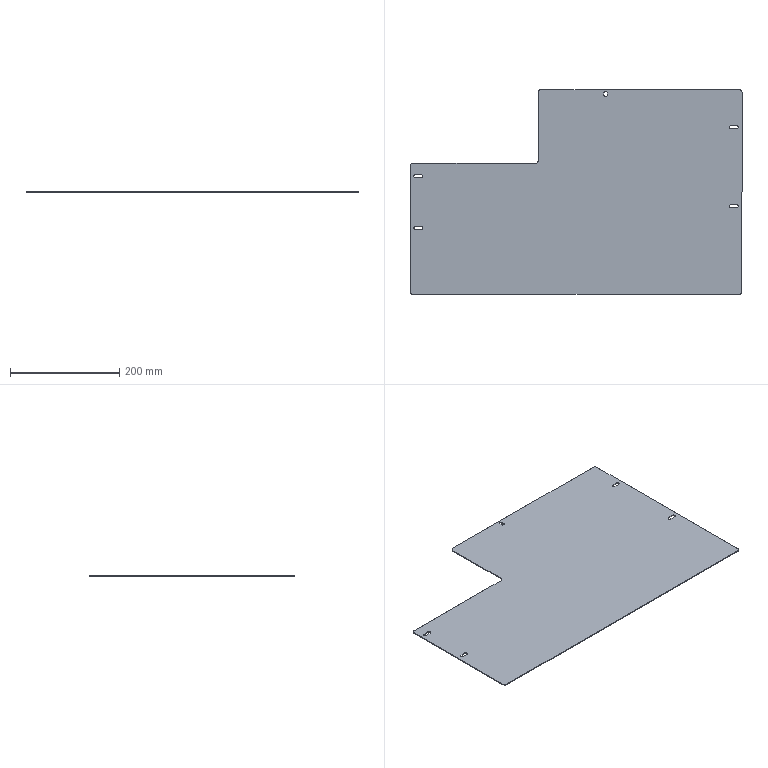Part | SolidWorks | features ICE 3, LPattern 2, FlatPattern 1, SMBaseFlange 1, SheetMetal 1 | 1 solid | 38 faces | box 608.5 x 375 x 1.5 mm | volume 294054 mm3 | cylinder 20 | plane 18 | commonest cylinder face diameters 6 x14 10 x6
STEP:
#1=CARTESIAN_POINT('',(755.768,60.78,-1.5));
#2=VERTEX_POINT('',#1);
#3=CARTESIAN_POINT('',(752.768,63.78,-1.5));
#4=VERTEX_POINT('',#3);
#5=CARTESIAN_POINT('',(752.768,60.78,-1.5));
#6=DIRECTION('',(0.,0.,1.));
#7=DIRECTION('',(1.,0.,0.));
#8=AXIS2_PLACEMENT_3D('',#5,#6,#7);
#9=CIRCLE('',#8,3.);
#10=EDGE_CURVE('',#2,#4,#9,.T.);
#11=ORIENTED_EDGE('',*,*,#10,.F.);
#12=CARTESIAN_POINT('',(755.768,60.78,0.));
#13=VERTEX_POINT('',#12);
#14=CARTESIAN_POINT('',(755.768,60.78,-1.5));
#15=DIRECTION('',(0.,0.,1.));
#16=VECTOR('',#15,1000.);
#17=LINE('',#14,#16);
#18=EDGE_CURVE('',#2,#13,#17,.T.);
#19=ORIENTED_EDGE('',*,*,#18,.T.);
#20=CARTESIAN_POINT('',(752.768,63.78,0.));
#21=VERTEX_POINT('',#20);
#22=CARTESIAN_POINT('',(752.768,60.78,0.));
#23=DIRECTION('',(0.,0.,1.));
#24=DIRECTION('',(1.,0.,0.));
#25=AXIS2_PLACEMENT_3D('',#22,#23,#24);
#26=CIRCLE('',#25,3.);
#27=EDGE_CURVE('',#13,#21,#26,.T.);
#28=ORIENTED_EDGE('',*,*,#27,.T.);
#29=CARTESIAN_POINT('',(752.768,63.78,-1.5));
#30=DIRECTION('',(0.,0.,1.));
#31=VECTOR('',#30,1000.);
#32=LINE('',#29,#31);
#33=EDGE_CURVE('',#4,#21,#32,.T.);
#34=ORIENTED_EDGE('',*,*,#33,.F.);
#35=EDGE_LOOP('',(#11,#19,#28,#34));
#36=FACE_OUTER_BOUND('',#35,.T.);
#37=CARTESIAN_POINT('',(752.768,60.78,-1.5));
#38=DIRECTION('',(0.,0.,1.));
#39=DIRECTION('',(1.,0.,0.));
#40=AXIS2_PLACEMENT_3D('',#37,#38,#39);
#41=CYLINDRICAL_SURFACE('',#40,3.);
#42=ADVANCED_FACE('',(#36),#41,.F.);
#43=CARTESIAN_POINT('',(755.768,205.78,-1.5));
#44=VERTEX_POINT('',#43);
#45=CARTESIAN_POINT('',(752.768,208.78,-1.5));
#46=VERTEX_POINT('',#45);
#47=CARTESIAN_POINT('',(752.768,205.78,-1.5));
#48=DIRECTION('',(0.,0.,1.));
#49=DIRECTION('',(1.,0.,0.));
#50=AXIS2_PLACEMENT_3D('',#47,#48,#49);
#51=CIRCLE('',#50,3.);
#52=EDGE_CURVE('',#44,#46,#51,.T.);
#53=ORIENTED_EDGE('',*,*,#52,.F.);
#54=CARTESIAN_POINT('',(755.768,205.78,0.));
#55=VERTEX_POINT('',#54);
#56=CARTESIAN_POINT('',(755.768,205.78,-1.5));
#57=DIRECTION('',(0.,0.,1.));
#58=VECTOR('',#57,1000.);
#59=LINE('',#56,#58);
#60=EDGE_CURVE('',#44,#55,#59,.T.);
#61=ORIENTED_EDGE('',*,*,#60,.T.);
#62=CARTESIAN_POINT('',(752.768,208.78,0.));
#63=VERTEX_POINT('',#62);
#64=CARTESIAN_POINT('',(752.768,205.78,0.));
#65=DIRECTION('',(0.,0.,1.));
#66=DIRECTION('',(1.,0.,0.));
#67=AXIS2_PLACEMENT_3D('',#64,#65,#66);
#68=CIRCLE('',#67,3.);
#69=EDGE_CURVE('',#55,#63,#68,.T.);
#70=ORIENTED_EDGE('',*,*,#69,.T.);
#71=CARTESIAN_POINT('',(752.768,208.78,-1.5));
#72=DIRECTION('',(0.,0.,1.));
#73=VECTOR('',#72,1000.);
#74=LINE('',#71,#73);
#75=EDGE_CURVE('',#46,#63,#74,.T.);
#76=ORIENTED_EDGE('',*,*,#75,.F.);
#77=EDGE_LOOP('',(#53,#61,#70,#76));
#78=FACE_OUTER_BOUND('',#77,.T.);
#79=CARTESIAN_POINT('',(752.768,205.78,-1.5));
#80=DIRECTION('',(0.,0.,1.));
#81=DIRECTION('',(1.,0.,0.));
#82=AXIS2_PLACEMENT_3D('',#79,#80,#81);
#83=CYLINDRICAL_SURFACE('',#82,3.);
#84=ADVANCED_FACE('',(#78),#83,.F.);
#85=CARTESIAN_POINT('',(174.268,118.78,-1.5));
#86=VERTEX_POINT('',#85);
#87=CARTESIAN_POINT('',(177.268,115.78,-1.5));
#88=VERTEX_POINT('',#87);
#89=CARTESIAN_POINT('',(174.268,115.78,-1.5));
#90=DIRECTION('',(0.,0.,-1.));
#91=DIRECTION('',(-1.,0.,0.));
#92=AXIS2_PLACEMENT_3D('',#89,#90,#91);
#93=CIRCLE('',#92,3.);
#94=EDGE_CURVE('',#86,#88,#93,.T.);
#95=ORIENTED_EDGE('',*,*,#94,.T.);
#96=CARTESIAN_POINT('',(177.268,115.78,0.));
#97=VERTEX_POINT('',#96);
#98=CARTESIAN_POINT('',(177.268,115.78,-10.));
#99=DIRECTION('',(0.,0.,1.));
#100=VECTOR('',#99,1000.);
#101=LINE('',#98,#100);
#102=EDGE_CURVE('',#88,#97,#101,.T.);
#103=ORIENTED_EDGE('',*,*,#102,.T.);
#104=CARTESIAN_POINT('',(174.268,118.78,0.));
#105=VERTEX_POINT('',#104);
#106=CARTESIAN_POINT('',(174.268,115.78,0.));
#107=DIRECTION('',(0.,0.,1.));
#108=DIRECTION('',(1.,0.,0.));
#109=AXIS2_PLACEMENT_3D('',#106,#107,#108);
#110=CIRCLE('',#109,3.);
#111=EDGE_CURVE('',#97,#105,#110,.T.);
#112=ORIENTED_EDGE('',*,*,#111,.T.);
#113=CARTESIAN_POINT('',(174.268,118.78,-10.));
#114=DIRECTION('',(0.,0.,1.));
#115=VECTOR('',#114,1000.);
#116=LINE('',#113,#115);
#117=EDGE_CURVE('',#86,#105,#116,.T.);
#118=ORIENTED_EDGE('',*,*,#117,.F.);
#119=EDGE_LOOP('',(#95,#103,#112,#118));
#120=FACE_OUTER_BOUND('',#119,.T.);
#121=CARTESIAN_POINT('',(174.268,115.78,-10.));
#122=DIRECTION('',(0.,0.,1.));
#123=DIRECTION('',(1.,0.,0.));
#124=AXIS2_PLACEMENT_3D('',#121,#122,#123);
#125=CYLINDRICAL_SURFACE('',#124,3.);
#126=ADVANCED_FACE('',(#120),#125,.F.);
#127=CARTESIAN_POINT('',(174.268,23.78,-1.5));
#128=VERTEX_POINT('',#127);
#129=CARTESIAN_POINT('',(177.268,20.78,-1.5));
#130=VERTEX_POINT('',#129);
#131=CARTESIAN_POINT('',(174.268,20.78,-1.5));
#132=DIRECTION('',(0.,0.,-1.));
#133=DIRECTION('',(-1.,0.,0.));
#134=AXIS2_PLACEMENT_3D('',#131,#132,#133);
#135=CIRCLE('',#134,3.);
#136=EDGE_CURVE('',#128,#130,#135,.T.);
#137=ORIENTED_EDGE('',*,*,#136,.T.);
#138=CARTESIAN_POINT('',(177.268,20.78,0.));
#139=VERTEX_POINT('',#138);
#140=CARTESIAN_POINT('',(177.268,20.78,-10.));
#141=DIRECTION('',(0.,0.,1.));
#142=VECTOR('',#141,1000.);
#143=LINE('',#140,#142);
#144=EDGE_CURVE('',#130,#139,#143,.T.);
#145=ORIENTED_EDGE('',*,*,#144,.T.);
#146=CARTESIAN_POINT('',(174.268,23.78,0.));
#147=VERTEX_POINT('',#146);
#148=CARTESIAN_POINT('',(174.268,20.78,0.));
#149=DIRECTION('',(0.,0.,1.));
#150=DIRECTION('',(1.,0.,0.));
#151=AXIS2_PLACEMENT_3D('',#148,#149,#150);
#152=CIRCLE('',#151,3.);
#153=EDGE_CURVE('',#139,#147,#152,.T.);
#154=ORIENTED_EDGE('',*,*,#153,.T.);
#155=CARTESIAN_POINT('',(174.268,23.78,-10.));
#156=DIRECTION('',(0.,0.,1.));
#157=VECTOR('',#156,1000.);
#158=LINE('',#155,#157);
#159=EDGE_CURVE('',#128,#147,#158,.T.);
#160=ORIENTED_EDGE('',*,*,#159,.F.);
#161=EDGE_LOOP('',(#137,#145,#154,#160));
#162=FACE_OUTER_BOUND('',#161,.T.);
#163=CARTESIAN_POINT('',(174.268,20.78,-10.));
#164=DIRECTION('',(0.,0.,1.));
#165=DIRECTION('',(1.,0.,0.));
#166=AXIS2_PLACEMENT_3D('',#163,#164,#165);
#167=CYLINDRICAL_SURFACE('',#166,3.);
#168=ADVANCED_FACE('',(#162),#167,.F.);
#169=CARTESIAN_POINT('',(389.268,144.28,0.));
#170=VERTEX_POINT('',#169);
#171=CARTESIAN_POINT('',(384.268,139.28,0.));
#172=VERTEX_POINT('',#171);
#173=CARTESIAN_POINT('',(384.268,144.28,0.));
#174=DIRECTION('',(0.,0.,-1.));
#175=DIRECTION('',(-1.,0.,0.));
#176=AXIS2_PLACEMENT_3D('',#173,#174,#175);
#177=CIRCLE('',#176,5.);
#178=EDGE_CURVE('',#170,#172,#177,.T.);
#179=ORIENTED_EDGE('',*,*,#178,.F.);
#180=CARTESIAN_POINT('',(389.268,144.28,-1.5));
#181=VERTEX_POINT('',#180);
#182=CARTESIAN_POINT('',(389.268,144.28,-1.5));
#183=DIRECTION('',(0.,0.,1.));
#184=VECTOR('',#183,1000.);
#185=LINE('',#182,#184);
#186=EDGE_CURVE('',#181,#170,#185,.T.);
#187=ORIENTED_EDGE('',*,*,#186,.F.);
#188=CARTESIAN_POINT('',(384.268,139.28,-1.5));
#189=VERTEX_POINT('',#188);
#190=CARTESIAN_POINT('',(384.268,144.28,-1.5));
#191=DIRECTION('',(0.,0.,-1.));
#192=DIRECTION('',(-1.,0.,0.));
#193=AXIS2_PLACEMENT_3D('',#190,#191,#192);
#194=CIRCLE('',#193,5.);
#195=EDGE_CURVE('',#181,#189,#194,.T.);
#196=ORIENTED_EDGE('',*,*,#195,.T.);
#197=CARTESIAN_POINT('',(384.268,139.28,-1.5));
#198=DIRECTION('',(0.,0.,1.));
#199=VECTOR('',#198,1000.);
#200=LINE('',#197,#199);
#201=EDGE_CURVE('',#189,#172,#200,.T.);
#202=ORIENTED_EDGE('',*,*,#201,.T.);
#203=EDGE_LOOP('',(#179,#187,#196,#202));
#204=FACE_OUTER_BOUND('',#203,.T.);
#205=CARTESIAN_POINT('',(384.268,144.28,-1.5));
#206=DIRECTION('',(0.,0.,1.));
#207=DIRECTION('',(1.,0.,0.));
#208=AXIS2_PLACEMENT_3D('',#205,#206,#207);
#209=CYLINDRICAL_SURFACE('',#208,5.);
#210=ADVANCED_FACE('',(#204),#209,.F.);
#211=CARTESIAN_POINT('',(389.268,269.28,0.));
#212=VERTEX_POINT('',#211);
#213=CARTESIAN_POINT('',(389.268,269.28,0.));
#214=DIRECTION('',(0.,-1.,0.));
#215=VECTOR('',#214,1000.);
#216=LINE('',#213,#215);
#217=EDGE_CURVE('',#212,#170,#216,.T.);
#218=ORIENTED_EDGE('',*,*,#217,.F.);
#219=CARTESIAN_POINT('',(389.268,269.28,-1.5));
#220=VERTEX_POINT('',#219);
#221=CARTESIAN_POINT('',(389.268,269.28,-1.5));
#222=DIRECTION('',(0.,0.,1.));
#223=VECTOR('',#222,1000.);
#224=LINE('',#221,#223);
#225=EDGE_CURVE('',#220,#212,#224,.T.);
#226=ORIENTED_EDGE('',*,*,#225,.F.);
#227=CARTESIAN_POINT('',(389.268,269.28,-1.5));
#228=DIRECTION('',(0.,-1.,0.));
#229=VECTOR('',#228,1000.);
#230=LINE('',#227,#229);
#231=EDGE_CURVE('',#220,#181,#230,.T.);
#232=ORIENTED_EDGE('',*,*,#231,.T.);
#233=ORIENTED_EDGE('',*,*,#186,.T.);
#234=EDGE_LOOP('',(#218,#226,#232,#233));
#235=FACE_OUTER_BOUND('',#234,.T.);
#236=CARTESIAN_POINT('',(389.268,269.28,-1.5));
#237=DIRECTION('',(-1.,0.,0.));
#238=DIRECTION('',(0.,0.,1.));
#239=AXIS2_PLACEMENT_3D('',#236,#237,#238);
#240=PLANE('',#239);
#241=ADVANCED_FACE('',(#235),#240,.T.);
#242=CARTESIAN_POINT('',(394.268,274.28,0.));
#243=VERTEX_POINT('',#242);
#244=CARTESIAN_POINT('',(394.268,269.28,0.));
#245=DIRECTION('',(0.,0.,1.));
#246=DIRECTION('',(-1.,0.,0.));
#247=AXIS2_PLACEMENT_3D('',#244,#245,#246);
#248=CIRCLE('',#247,5.);
#249=EDGE_CURVE('',#243,#212,#248,.T.);
#250=ORIENTED_EDGE('',*,*,#249,.F.);
#251=CARTESIAN_POINT('',(394.268,274.28,-1.5));
#252=VERTEX_POINT('',#251);
#253=CARTESIAN_POINT('',(394.268,274.28,-1.5));
#254=DIRECTION('',(0.,0.,1.));
#255=VECTOR('',#254,1000.);
#256=LINE('',#253,#255);
#257=EDGE_CURVE('',#252,#243,#256,.T.);
#258=ORIENTED_EDGE('',*,*,#257,.F.);
#259=CARTESIAN_POINT('',(394.268,269.28,-1.5));
#260=DIRECTION('',(0.,0.,1.));
#261=DIRECTION('',(-1.,0.,0.));
#262=AXIS2_PLACEMENT_3D('',#259,#260,#261);
#263=CIRCLE('',#262,5.);
#264=EDGE_CURVE('',#252,#220,#263,.T.);
#265=ORIENTED_EDGE('',*,*,#264,.T.);
#266=ORIENTED_EDGE('',*,*,#225,.T.);
#267=EDGE_LOOP('',(#250,#258,#265,#266));
#268=FACE_OUTER_BOUND('',#267,.T.);
#269=CARTESIAN_POINT('',(394.268,269.28,-1.5));
#270=DIRECTION('',(0.,0.,1.));
#271=DIRECTION('',(1.,0.,0.));
#272=AXIS2_PLACEMENT_3D('',#269,#270,#271);
#273=CYLINDRICAL_SURFACE('',#272,5.);
#274=ADVANCED_FACE('',(#268),#273,.T.);
#275=CARTESIAN_POINT('',(757.768,274.28,0.));
#276=VERTEX_POINT('',#275);
#277=CARTESIAN_POINT('',(757.768,274.28,0.));
#278=DIRECTION('',(-1.,0.,0.));
#279=VECTOR('',#278,1000.);
#280=LINE('',#277,#279);
#281=EDGE_CURVE('',#276,#243,#280,.T.);
#282=ORIENTED_EDGE('',*,*,#281,.F.);
#283=CARTESIAN_POINT('',(757.768,274.28,-1.5));
#284=VERTEX_POINT('',#283);
#285=CARTESIAN_POINT('',(757.768,274.28,-1.5));
#286=DIRECTION('',(0.,0.,1.));
#287=VECTOR('',#286,1000.);
#288=LINE('',#285,#287);
#289=EDGE_CURVE('',#284,#276,#288,.T.);
#290=ORIENTED_EDGE('',*,*,#289,.F.);
#291=CARTESIAN_POINT('',(757.768,274.28,-1.5));
#292=DIRECTION('',(-1.,0.,0.));
#293=VECTOR('',#292,1000.);
#294=LINE('',#291,#293);
#295=EDGE_CURVE('',#284,#252,#294,.T.);
#296=ORIENTED_EDGE('',*,*,#295,.T.);
#297=ORIENTED_EDGE('',*,*,#257,.T.);
#298=EDGE_LOOP('',(#282,#290,#296,#297));
#299=FACE_OUTER_BOUND('',#298,.T.);
#300=CARTESIAN_POINT('',(757.768,274.28,-1.5));
#301=DIRECTION('',(0.,1.,0.));
#302=DIRECTION('',(0.,0.,1.));
#303=AXIS2_PLACEMENT_3D('',#300,#301,#302);
#304=PLANE('',#303);
#305=ADVANCED_FACE('',(#299),#304,.T.);
#306=CARTESIAN_POINT('',(762.768,269.28,0.));
#307=VERTEX_POINT('',#306);
#308=CARTESIAN_POINT('',(757.768,269.28,0.));
#309=DIRECTION('',(0.,0.,1.));
#310=DIRECTION('',(1.,0.,0.));
#311=AXIS2_PLACEMENT_3D('',#308,#309,#310);
#312=CIRCLE('',#311,5.);
#313=EDGE_CURVE('',#307,#276,#312,.T.);
#314=ORIENTED_EDGE('',*,*,#313,.F.);
#315=CARTESIAN_POINT('',(762.768,269.28,-1.5));
#316=VERTEX_POINT('',#315);
#317=CARTESIAN_POINT('',(762.768,269.28,-1.5));
#318=DIRECTION('',(0.,0.,1.));
#319=VECTOR('',#318,1000.);
#320=LINE('',#317,#319);
#321=EDGE_CURVE('',#316,#307,#320,.T.);
#322=ORIENTED_EDGE('',*,*,#321,.F.);
#323=CARTESIAN_POINT('',(757.768,269.28,-1.5));
#324=DIRECTION('',(0.,0.,1.));
#325=DIRECTION('',(1.,0.,0.));
#326=AXIS2_PLACEMENT_3D('',#323,#324,#325);
#327=CIRCLE('',#326,5.);
#328=EDGE_CURVE('',#316,#284,#327,.T.);
#329=ORIENTED_EDGE('',*,*,#328,.T.);
#330=ORIENTED_EDGE('',*,*,#289,.T.);
#331=EDGE_LOOP('',(#314,#322,#329,#330));
#332=FACE_OUTER_BOUND('',#331,.T.);
#333=CARTESIAN_POINT('',(757.768,269.28,-1.5));
#334=DIRECTION('',(0.,0.,1.));
#335=DIRECTION('',(1.,0.,0.));
#336=AXIS2_PLACEMENT_3D('',#333,#334,#335);
#337=CYLINDRICAL_SURFACE('',#336,5.);
#338=ADVANCED_FACE('',(#332),#337,.T.);
#339=CARTESIAN_POINT('',(762.768,-95.72,0.));
#340=VERTEX_POINT('',#339);
#341=CARTESIAN_POINT('',(762.768,-95.72,0.));
#342=DIRECTION('',(0.,1.,0.));
#343=VECTOR('',#342,1000.);
#344=LINE('',#341,#343);
#345=EDGE_CURVE('',#340,#307,#344,.T.);
#346=ORIENTED_EDGE('',*,*,#345,.F.);
#347=CARTESIAN_POINT('',(762.768,-95.72,-1.5));
#348=VERTEX_POINT('',#347);
#349=CARTESIAN_POINT('',(762.768,-95.72,-1.5));
#350=DIRECTION('',(0.,0.,1.));
#351=VECTOR('',#350,1000.);
#352=LINE('',#349,#351);
#353=EDGE_CURVE('',#348,#340,#352,.T.);
#354=ORIENTED_EDGE('',*,*,#353,.F.);
#355=CARTESIAN_POINT('',(762.768,-95.72,-1.5));
#356=DIRECTION('',(0.,1.,0.));
#357=VECTOR('',#356,1000.);
#358=LINE('',#355,#357);
#359=EDGE_CURVE('',#348,#316,#358,.T.);
#360=ORIENTED_EDGE('',*,*,#359,.T.);
#361=ORIENTED_EDGE('',*,*,#321,.T.);
#362=EDGE_LOOP('',(#346,#354,#360,#361));
#363=FACE_OUTER_BOUND('',#362,.T.);
#364=CARTESIAN_POINT('',(762.768,-95.72,-1.5));
#365=DIRECTION('',(1.,0.,0.));
#366=DIRECTION('',(0.,1.,0.));
#367=AXIS2_PLACEMENT_3D('',#364,#365,#366);
#368=PLANE('',#367);
#369=ADVANCED_FACE('',(#363),#368,.T.);
#370=CARTESIAN_POINT('',(757.768,-100.72,0.));
#371=VERTEX_POINT('',#370);
#372=CARTESIAN_POINT('',(757.768,-95.72,0.));
#373=DIRECTION('',(0.,0.,1.));
#374=DIRECTION('',(-1.,0.,0.));
#375=AXIS2_PLACEMENT_3D('',#372,#373,#374);
#376=CIRCLE('',#375,5.);
#377=EDGE_CURVE('',#371,#340,#376,.T.);
#378=ORIENTED_EDGE('',*,*,#377,.F.);
#379=CARTESIAN_POINT('',(757.768,-100.72,-1.5));
#380=VERTEX_POINT('',#379);
#381=CARTESIAN_POINT('',(757.768,-100.72,-1.5));
#382=DIRECTION('',(0.,0.,1.));
#383=VECTOR('',#382,1000.);
#384=LINE('',#381,#383);
#385=EDGE_CURVE('',#380,#371,#384,.T.);
#386=ORIENTED_EDGE('',*,*,#385,.F.);
#387=CARTESIAN_POINT('',(757.768,-95.72,-1.5));
#388=DIRECTION('',(0.,0.,1.));
#389=DIRECTION('',(-1.,0.,0.));
#390=AXIS2_PLACEMENT_3D('',#387,#388,#389);
#391=CIRCLE('',#390,5.);
#392=EDGE_CURVE('',#380,#348,#391,.T.);
#393=ORIENTED_EDGE('',*,*,#392,.T.);
#394=ORIENTED_EDGE('',*,*,#353,.T.);
#395=EDGE_LOOP('',(#378,#386,#393,#394));
#396=FACE_OUTER_BOUND('',#395,.T.);
#397=CARTESIAN_POINT('',(757.768,-95.72,-1.5));
#398=DIRECTION('',(0.,0.,1.));
#399=DIRECTION('',(1.,0.,0.));
#400=AXIS2_PLACEMENT_3D('',#397,#398,#399);
#401=CYLINDRICAL_SURFACE('',#400,5.);
#402=ADVANCED_FACE('',(#396),#401,.T.);
#403=CARTESIAN_POINT('',(159.268,-100.72,0.));
#404=VERTEX_POINT('',#403);
#405=CARTESIAN_POINT('',(159.268,-100.72,0.));
#406=DIRECTION('',(1.,0.,0.));
#407=VECTOR('',#406,1000.);
#408=LINE('',#405,#407);
#409=EDGE_CURVE('',#404,#371,#408,.T.);
#410=ORIENTED_EDGE('',*,*,#409,.F.);
#411=CARTESIAN_POINT('',(159.268,-100.72,-1.5));
#412=VERTEX_POINT('',#411);
#413=CARTESIAN_POINT('',(159.268,-100.72,-1.5));
#414=DIRECTION('',(0.,0.,1.));
#415=VECTOR('',#414,1000.);
#416=LINE('',#413,#415);
#417=EDGE_CURVE('',#412,#404,#416,.T.);
#418=ORIENTED_EDGE('',*,*,#417,.F.);
#419=CARTESIAN_POINT('',(159.268,-100.72,-1.5));
#420=DIRECTION('',(1.,0.,0.));
#421=VECTOR('',#420,1000.);
#422=LINE('',#419,#421);
#423=EDGE_CURVE('',#412,#380,#422,.T.);
#424=ORIENTED_EDGE('',*,*,#423,.T.);
#425=ORIENTED_EDGE('',*,*,#385,.T.);
#426=EDGE_LOOP('',(#410,#418,#424,#425));
#427=FACE_OUTER_BOUND('',#426,.T.);
#428=CARTESIAN_POINT('',(159.268,-100.72,-1.5));
#429=DIRECTION('',(0.,-1.,0.));
#430=DIRECTION('',(0.,0.,-1.));
#431=AXIS2_PLACEMENT_3D('',#428,#429,#430);
#432=PLANE('',#431);
#433=ADVANCED_FACE('',(#427),#432,.T.);
#434=CARTESIAN_POINT('',(154.268,-95.72,0.));
#435=VERTEX_POINT('',#434);
#436=CARTESIAN_POINT('',(159.268,-95.72,0.));
#437=DIRECTION('',(0.,0.,1.));
#438=DIRECTION('',(-1.,0.,0.));
#439=AXIS2_PLACEMENT_3D('',#436,#437,#438);
#440=CIRCLE('',#439,5.);
#441=EDGE_CURVE('',#435,#404,#440,.T.);
#442=ORIENTED_EDGE('',*,*,#441,.F.);
#443=CARTESIAN_POINT('',(154.268,-95.72,-1.5));
#444=VERTEX_POINT('',#443);
#445=CARTESIAN_POINT('',(154.268,-95.72,-1.5));
#446=DIRECTION('',(0.,0.,1.));
#447=VECTOR('',#446,1000.);
#448=LINE('',#445,#447);
#449=EDGE_CURVE('',#444,#435,#448,.T.);
#450=ORIENTED_EDGE('',*,*,#449,.F.);
#451=CARTESIAN_POINT('',(159.268,-95.72,-1.5));
#452=DIRECTION('',(0.,0.,1.));
#453=DIRECTION('',(-1.,0.,0.));
#454=AXIS2_PLACEMENT_3D('',#451,#452,#453);
#455=CIRCLE('',#454,5.);
#456=EDGE_CURVE('',#444,#412,#455,.T.);
#457=ORIENTED_EDGE('',*,*,#456,.T.);
#458=ORIENTED_EDGE('',*,*,#417,.T.);
#459=EDGE_LOOP('',(#442,#450,#457,#458));
#460=FACE_OUTER_BOUND('',#459,.T.);
#461=CARTESIAN_POINT('',(159.268,-95.72,-1.5));
#462=DIRECTION('',(0.,0.,1.));
#463=DIRECTION('',(1.,0.,0.));
#464=AXIS2_PLACEMENT_3D('',#461,#462,#463);
#465=CYLINDRICAL_SURFACE('',#464,5.);
#466=ADVANCED_FACE('',(#460),#465,.T.);
#467=CARTESIAN_POINT('',(154.268,134.28,0.));
#468=VERTEX_POINT('',#467);
#469=CARTESIAN_POINT('',(154.268,134.28,0.));
#470=DIRECTION('',(0.,-1.,0.));
#471=VECTOR('',#470,1000.);
#472=LINE('',#469,#471);
#473=EDGE_CURVE('',#468,#435,#472,.T.);
#474=ORIENTED_EDGE('',*,*,#473,.F.);
#475=CARTESIAN_POINT('',(154.268,134.28,-1.5));
#476=VERTEX_POINT('',#475);
#477=CARTESIAN_POINT('',(154.268,134.28,-1.5));
#478=DIRECTION('',(0.,0.,1.));
#479=VECTOR('',#478,1000.);
#480=LINE('',#477,#479);
#481=EDGE_CURVE('',#476,#468,#480,.T.);
#482=ORIENTED_EDGE('',*,*,#481,.F.);
#483=CARTESIAN_POINT('',(154.268,134.28,-1.5));
#484=DIRECTION('',(0.,-1.,0.));
#485=VECTOR('',#484,1000.);
#486=LINE('',#483,#485);
#487=EDGE_CURVE('',#476,#444,#486,.T.);
#488=ORIENTED_EDGE('',*,*,#487,.T.);
#489=ORIENTED_EDGE('',*,*,#449,.T.);
#490=EDGE_LOOP('',(#474,#482,#488,#489));
#491=FACE_OUTER_BOUND('',#490,.T.);
#492=CARTESIAN_POINT('',(154.268,134.28,-1.5));
#493=DIRECTION('',(-1.,0.,0.));
#494=DIRECTION('',(0.,0.,1.));
#495=AXIS2_PLACEMENT_3D('',#492,#493,#494);
#496=PLANE('',#495);
#497=ADVANCED_FACE('',(#491),#496,.T.);
#498=CARTESIAN_POINT('',(159.268,139.28,0.));
#499=VERTEX_POINT('',#498);
#500=CARTESIAN_POINT('',(159.268,134.28,0.));
#501=DIRECTION('',(0.,0.,1.));
#502=DIRECTION('',(1.,0.,0.));
#503=AXIS2_PLACEMENT_3D('',#500,#501,#502);
#504=CIRCLE('',#503,5.);
#505=EDGE_CURVE('',#499,#468,#504,.T.);
#506=ORIENTED_EDGE('',*,*,#505,.F.);
#507=CARTESIAN_POINT('',(159.268,139.28,-1.5));
#508=VERTEX_POINT('',#507);
#509=CARTESIAN_POINT('',(159.268,139.28,-1.5));
#510=DIRECTION('',(0.,0.,1.));
#511=VECTOR('',#510,1000.);
#512=LINE('',#509,#511);
#513=EDGE_CURVE('',#508,#499,#512,.T.);
#514=ORIENTED_EDGE('',*,*,#513,.F.);
#515=CARTESIAN_POINT('',(159.268,134.28,-1.5));
#516=DIRECTION('',(0.,0.,1.));
#517=DIRECTION('',(1.,0.,0.));
#518=AXIS2_PLACEMENT_3D('',#515,#516,#517);
#519=CIRCLE('',#518,5.);
#520=EDGE_CURVE('',#508,#476,#519,.T.);
#521=ORIENTED_EDGE('',*,*,#520,.T.);
#522=ORIENTED_EDGE('',*,*,#481,.T.);
#523=EDGE_LOOP('',(#506,#514,#521,#522));
#524=FACE_OUTER_BOUND('',#523,.T.);
#525=CARTESIAN_POINT('',(159.268,134.28,-1.5));
#526=DIRECTION('',(0.,0.,1.));
#527=DIRECTION('',(1.,0.,0.));
#528=AXIS2_PLACEMENT_3D('',#525,#526,#527);
#529=CYLINDRICAL_SURFACE('',#528,5.);
#530=ADVANCED_FACE('',(#524),#529,.T.);
#531=CARTESIAN_POINT('',(384.268,139.28,0.));
#532=DIRECTION('',(-1.,0.,0.));
#533=VECTOR('',#532,1000.);
#534=LINE('',#531,#533);
#535=EDGE_CURVE('',#172,#499,#534,.T.);
#536=ORIENTED_EDGE('',*,*,#535,.F.);
#537=ORIENTED_EDGE('',*,*,#201,.F.);
#538=CARTESIAN_POINT('',(384.268,139.28,-1.5));
#539=DIRECTION('',(-1.,0.,0.));
#540=VECTOR('',#539,1000.);
#541=LINE('',#538,#540);
#542=EDGE_CURVE('',#189,#508,#541,.T.);
#543=ORIENTED_EDGE('',*,*,#542,.T.);
#544=ORIENTED_EDGE('',*,*,#513,.T.);
#545=EDGE_LOOP('',(#536,#537,#543,#544));
#546=FACE_OUTER_BOUND('',#545,.T.);
#547=CARTESIAN_POINT('',(384.268,139.28,-1.5));
#548=DIRECTION('',(0.,1.,0.));
#549=DIRECTION('',(-1.,0.,0.));
#550=AXIS2_PLACEMENT_3D('',#547,#548,#549);
#551=PLANE('',#550);
#552=ADVANCED_FACE('',(#546),#551,.T.);
#553=CARTESIAN_POINT('',(742.768,63.78,-1.5));
#554=VERTEX_POINT('',#553);
#555=CARTESIAN_POINT('',(742.768,57.78,-1.5));
#556=VERTEX_POINT('',#555);
#557=CARTESIAN_POINT('',(742.768,60.78,-1.5));
#558=DIRECTION('',(0.,0.,1.));
#559=DIRECTION('',(1.,0.,0.));
#560=AXIS2_PLACEMENT_3D('',#557,#558,#559);
#561=CIRCLE('',#560,3.);
#562=EDGE_CURVE('',#554,#556,#561,.T.);
#563=ORIENTED_EDGE('',*,*,#562,.T.);
#564=CARTESIAN_POINT('',(752.768,57.78,-1.5));
#565=VERTEX_POINT('',#564);
#566=CARTESIAN_POINT('',(742.768,57.78,-1.5));
#567=DIRECTION('',(1.,0.,0.));
#568=VECTOR('',#567,1000.);
#569=LINE('',#566,#568);
#570=EDGE_CURVE('',#556,#565,#569,.T.);
#571=ORIENTED_EDGE('',*,*,#570,.T.);
#572=CARTESIAN_POINT('',(752.768,60.78,-1.5));
#573=DIRECTION('',(0.,0.,1.));
#574=DIRECTION('',(1.,0.,0.));
#575=AXIS2_PLACEMENT_3D('',#572,#573,#574);
#576=CIRCLE('',#575,3.);
#577=EDGE_CURVE('',#565,#2,#576,.T.);
#578=ORIENTED_EDGE('',*,*,#577,.T.);
#579=ORIENTED_EDGE('',*,*,#10,.T.);
#580=CARTESIAN_POINT('',(742.768,63.78,-1.5));
#581=DIRECTION('',(-1.,0.,0.));
#582=VECTOR('',#581,1000.);
#583=LINE('',#580,#582);
#584=EDGE_CURVE('',#4,#554,#583,.T.);
#585=ORIENTED_EDGE('',*,*,#584,.T.);
#586=EDGE_LOOP('',(#563,#571,#578,#579,#585));
#587=FACE_BOUND('',#586,.T.);
#588=CARTESIAN_POINT('',(742.768,208.78,-1.5));
#589=VERTEX_POINT('',#588);
#590=CARTESIAN_POINT('',(742.768,202.78,-1.5));
#591=VERTEX_POINT('',#590);
#592=CARTESIAN_POINT('',(742.768,205.78,-1.5));
#593=DIRECTION('',(0.,0.,1.));
#594=DIRECTION('',(1.,0.,0.));
#595=AXIS2_PLACEMENT_3D('',#592,#593,#594);
#596=CIRCLE('',#595,3.);
#597=EDGE_CURVE('',#589,#591,#596,.T.);
#598=ORIENTED_EDGE('',*,*,#597,.T.);
#599=CARTESIAN_POINT('',(752.768,202.78,-1.5));
#600=VERTEX_POINT('',#599);
#601=CARTESIAN_POINT('',(742.768,202.78,-1.5));
#602=DIRECTION('',(1.,0.,0.));
#603=VECTOR('',#602,1000.);
#604=LINE('',#601,#603);
#605=EDGE_CURVE('',#591,#600,#604,.T.);
#606=ORIENTED_EDGE('',*,*,#605,.T.);
#607=CARTESIAN_POINT('',(752.768,205.78,-1.5));
#608=DIRECTION('',(0.,0.,1.));
#609=DIRECTION('',(1.,0.,0.));
#610=AXIS2_PLACEMENT_3D('',#607,#608,#609);
#611=CIRCLE('',#610,3.);
#612=EDGE_CURVE('',#600,#44,#611,.T.);
#613=ORIENTED_EDGE('',*,*,#612,.T.);
#614=ORIENTED_EDGE('',*,*,#52,.T.);
#615=CARTESIAN_POINT('',(742.768,208.78,-1.5));
#616=DIRECTION('',(-1.,0.,0.));
#617=VECTOR('',#616,1000.);
#618=LINE('',#615,#617);
#619=EDGE_CURVE('',#46,#589,#618,.T.);
#620=ORIENTED_EDGE('',*,*,#619,.T.);
#621=EDGE_LOOP('',(#598,#606,#613,#614,#620));
#622=FACE_BOUND('',#621,.T.);
#623=CARTESIAN_POINT('',(509.768,268.28,-1.5));
#624=VERTEX_POINT('',#623);
#625=CARTESIAN_POINT('',(515.768,268.28,-1.5));
#626=VERTEX_POINT('',#625);
#627=CARTESIAN_POINT('',(512.768,268.28,-1.5));
#628=DIRECTION('',(0.,0.,-1.));
#629=DIRECTION('',(-1.,0.,0.));
#630=AXIS2_PLACEMENT_3D('',#627,#628,#629);
#631=CIRCLE('',#630,3.);
#632=EDGE_CURVE('',#624,#626,#631,.T.);
#633=ORIENTED_EDGE('',*,*,#632,.F.);
#634=CARTESIAN_POINT('',(509.768,264.28,-1.5));
#635=VERTEX_POINT('',#634);
#636=CARTESIAN_POINT('',(509.768,144.28,-1.5));
#637=DIRECTION('',(0.,1.,0.));
#638=VECTOR('',#637,1000.);
#639=LINE('',#636,#638);
#640=EDGE_CURVE('',#635,#624,#639,.T.);
#641=ORIENTED_EDGE('',*,*,#640,.F.);
#642=CARTESIAN_POINT('',(515.768,264.28,-1.5));
#643=VERTEX_POINT('',#642);
#644=CARTESIAN_POINT('',(512.768,264.28,-1.5));
#645=DIRECTION('',(0.,0.,-1.));
#646=DIRECTION('',(-1.,0.,0.));
#647=AXIS2_PLACEMENT_3D('',#644,#645,#646);
#648=CIRCLE('',#647,3.);
#649=EDGE_CURVE('',#643,#635,#648,.T.);
#650=ORIENTED_EDGE('',*,*,#649,.F.);
#651=CARTESIAN_POINT('',(515.768,144.28,-1.5));
#652=DIRECTION('',(0.,-1.,0.));
#653=VECTOR('',#652,1000.);
#654=LINE('',#651,#653);
#655=EDGE_CURVE('',#626,#643,#654,.T.);
#656=ORIENTED_EDGE('',*,*,#655,.F.);
#657=EDGE_LOOP('',(#633,#641,#650,#656));
#658=FACE_BOUND('',#657,.T.);
#659=CARTESIAN_POINT('',(164.268,112.78,-1.5));
#660=VERTEX_POINT('',#659);
#661=CARTESIAN_POINT('',(164.268,118.78,-1.5));
#662=VERTEX_POINT('',#661);
#663=CARTESIAN_POINT('',(164.268,115.78,-1.5));
#664=DIRECTION('',(0.,0.,-1.));
#665=DIRECTION('',(-1.,0.,0.));
#666=AXIS2_PLACEMENT_3D('',#663,#664,#665);
#667=CIRCLE('',#666,3.);
#668=EDGE_CURVE('',#660,#662,#667,.T.);
#669=ORIENTED_EDGE('',*,*,#668,.F.);
#670=CARTESIAN_POINT('',(174.268,112.78,-1.5));
#671=VERTEX_POINT('',#670);
#672=CARTESIAN_POINT('',(384.268,112.78,-1.5));
#673=DIRECTION('',(-1.,0.,0.));
#674=VECTOR('',#673,1000.);
#675=LINE('',#672,#674);
#676=EDGE_CURVE('',#671,#660,#675,.T.);
#677=ORIENTED_EDGE('',*,*,#676,.F.);
#678=CARTESIAN_POINT('',(174.268,115.78,-1.5));
#679=DIRECTION('',(0.,0.,-1.));
#680=DIRECTION('',(-1.,0.,0.));
#681=AXIS2_PLACEMENT_3D('',#678,#679,#680);
#682=CIRCLE('',#681,3.);
#683=EDGE_CURVE('',#88,#671,#682,.T.);
#684=ORIENTED_EDGE('',*,*,#683,.F.);
#685=ORIENTED_EDGE('',*,*,#94,.F.);
#686=CARTESIAN_POINT('',(384.268,118.78,-1.5));
#687=DIRECTION('',(1.,0.,0.));
#688=VECTOR('',#687,1000.);
#689=LINE('',#686,#688);
#690=EDGE_CURVE('',#662,#86,#689,.T.);
#691=ORIENTED_EDGE('',*,*,#690,.F.);
#692=EDGE_LOOP('',(#669,#677,#684,#685,#691));
#693=FACE_BOUND('',#692,.T.);
#694=CARTESIAN_POINT('',(164.268,17.78,-1.5));
#695=VERTEX_POINT('',#694);
#696=CARTESIAN_POINT('',(164.268,23.78,-1.5));
#697=VERTEX_POINT('',#696);
#698=CARTESIAN_POINT('',(164.268,20.78,-1.5));
#699=DIRECTION('',(0.,0.,-1.));
#700=DIRECTION('',(-1.,0.,0.));
#701=AXIS2_PLACEMENT_3D('',#698,#699,#700);
#702=CIRCLE('',#701,3.);
#703=EDGE_CURVE('',#695,#697,#702,.T.);
#704=ORIENTED_EDGE('',*,*,#703,.F.);
#705=CARTESIAN_POINT('',(174.268,17.78,-1.5));
#706=VERTEX_POINT('',#705);
#707=CARTESIAN_POINT('',(384.268,17.78,-1.5));
#708=DIRECTION('',(-1.,0.,0.));
#709=VECTOR('',#708,1000.);
#710=LINE('',#707,#709);
#711=EDGE_CURVE('',#706,#695,#710,.T.);
#712=ORIENTED_EDGE('',*,*,#711,.F.);
#713=CARTESIAN_POINT('',(174.268,20.78,-1.5));
#714=DIRECTION('',(0.,0.,-1.));
#715=DIRECTION('',(-1.,0.,0.));
#716=AXIS2_PLACEMENT_3D('',#713,#714,#715);
#717=CIRCLE('',#716,3.);
#718=EDGE_CURVE('',#130,#706,#717,.T.);
#719=ORIENTED_EDGE('',*,*,#718,.F.);
#720=ORIENTED_EDGE('',*,*,#136,.F.);
#721=CARTESIAN_POINT('',(384.268,23.78,-1.5));
#722=DIRECTION('',(1.,0.,0.));
#723=VECTOR('',#722,1000.);
#724=LINE('',#721,#723);
#725=EDGE_CURVE('',#697,#128,#724,.T.);
#726=ORIENTED_EDGE('',*,*,#725,.F.);
#727=EDGE_LOOP('',(#704,#712,#719,#720,#726));
#728=FACE_BOUND('',#727,.T.);
#729=ORIENTED_EDGE('',*,*,#195,.F.);
#730=ORIENTED_EDGE('',*,*,#231,.F.);
#731=ORIENTED_EDGE('',*,*,#264,.F.);
#732=ORIENTED_EDGE('',*,*,#295,.F.);
#733=ORIENTED_EDGE('',*,*,#328,.F.);
#734=ORIENTED_EDGE('',*,*,#359,.F.);
#735=ORIENTED_EDGE('',*,*,#392,.F.);
#736=ORIENTED_EDGE('',*,*,#423,.F.);
#737=ORIENTED_EDGE('',*,*,#456,.F.);
#738=ORIENTED_EDGE('',*,*,#487,.F.);
#739=ORIENTED_EDGE('',*,*,#520,.F.);
#740=ORIENTED_EDGE('',*,*,#542,.F.);
#741=EDGE_LOOP('',(#729,#730,#731,#732,#733,#734,#735,#736,#737,#738,#739,#740));
#742=FACE_OUTER_BOUND('',#741,.T.);
#743=CARTESIAN_POINT('',(384.268,144.28,-1.5));
#744=DIRECTION('',(0.,0.,-1.));
#745=DIRECTION('',(-1.,0.,0.));
#746=AXIS2_PLACEMENT_3D('',#743,#744,#745);
#747=PLANE('',#746);
#748=ADVANCED_FACE('',(#587,#622,#658,#693,#728,#742),#747,.T.);
#749=CARTESIAN_POINT('',(742.768,57.78,0.));
#750=VERTEX_POINT('',#749);
#751=CARTESIAN_POINT('',(752.768,57.78,0.));
#752=VERTEX_POINT('',#751);
#753=CARTESIAN_POINT('',(742.768,57.78,0.));
#754=DIRECTION('',(1.,0.,0.));
#755=VECTOR('',#754,1000.);
#756=LINE('',#753,#755);
#757=EDGE_CURVE('',#750,#752,#756,.T.);
#758=ORIENTED_EDGE('',*,*,#757,.F.);
#759=CARTESIAN_POINT('',(742.768,63.78,0.));
#760=VERTEX_POINT('',#759);
#761=CARTESIAN_POINT('',(742.768,60.78,0.));
#762=DIRECTION('',(0.,0.,1.));
#763=DIRECTION('',(1.,0.,0.));
#764=AXIS2_PLACEMENT_3D('',#761,#762,#763);
#765=CIRCLE('',#764,3.);
#766=EDGE_CURVE('',#760,#750,#765,.T.);
#767=ORIENTED_EDGE('',*,*,#766,.F.);
#768=CARTESIAN_POINT('',(742.768,63.78,0.));
#769=DIRECTION('',(-1.,0.,0.));
#770=VECTOR('',#769,1000.);
#771=LINE('',#768,#770);
#772=EDGE_CURVE('',#21,#760,#771,.T.);
#773=ORIENTED_EDGE('',*,*,#772,.F.);
#774=ORIENTED_EDGE('',*,*,#27,.F.);
#775=CARTESIAN_POINT('',(752.768,60.78,0.));
#776=DIRECTION('',(0.,0.,1.));
#777=DIRECTION('',(1.,0.,0.));
#778=AXIS2_PLACEMENT_3D('',#775,#776,#777);
#779=CIRCLE('',#778,3.);
#780=EDGE_CURVE('',#752,#13,#779,.T.);
#781=ORIENTED_EDGE('',*,*,#780,.F.);
#782=EDGE_LOOP('',(#758,#767,#773,#774,#781));
#783=FACE_BOUND('',#782,.T.);
#784=CARTESIAN_POINT('',(742.768,202.78,0.));
#785=VERTEX_POINT('',#784);
#786=CARTESIAN_POINT('',(752.768,202.78,0.));
#787=VERTEX_POINT('',#786);
#788=CARTESIAN_POINT('',(742.768,202.78,0.));
#789=DIRECTION('',(1.,0.,0.));
#790=VECTOR('',#789,1000.);
#791=LINE('',#788,#790);
#792=EDGE_CURVE('',#785,#787,#791,.T.);
#793=ORIENTED_EDGE('',*,*,#792,.F.);
#794=CARTESIAN_POINT('',(742.768,208.78,0.));
#795=VERTEX_POINT('',#794);
#796=CARTESIAN_POINT('',(742.768,205.78,0.));
#797=DIRECTION('',(0.,0.,1.));
#798=DIRECTION('',(1.,0.,0.));
#799=AXIS2_PLACEMENT_3D('',#796,#797,#798);
#800=CIRCLE('',#799,3.);
#801=EDGE_CURVE('',#795,#785,#800,.T.);
#802=ORIENTED_EDGE('',*,*,#801,.F.);
#803=CARTESIAN_POINT('',(742.768,208.78,0.));
#804=DIRECTION('',(-1.,0.,0.));
#805=VECTOR('',#804,1000.);
#806=LINE('',#803,#805);
#807=EDGE_CURVE('',#63,#795,#806,.T.);
#808=ORIENTED_EDGE('',*,*,#807,.F.);
#809=ORIENTED_EDGE('',*,*,#69,.F.);
#810=CARTESIAN_POINT('',(752.768,205.78,0.));
#811=DIRECTION('',(0.,0.,1.));
#812=DIRECTION('',(1.,0.,0.));
#813=AXIS2_PLACEMENT_3D('',#810,#811,#812);
#814=CIRCLE('',#813,3.);
#815=EDGE_CURVE('',#787,#55,#814,.T.);
#816=ORIENTED_EDGE('',*,*,#815,.F.);
#817=EDGE_LOOP('',(#793,#802,#808,#809,#816));
#818=FACE_BOUND('',#817,.T.);
#819=CARTESIAN_POINT('',(509.768,268.28,0.));
#820=VERTEX_POINT('',#819);
#821=CARTESIAN_POINT('',(509.768,264.28,0.));
#822=VERTEX_POINT('',#821);
#823=CARTESIAN_POINT('',(509.768,268.28,0.));
#824=DIRECTION('',(0.,-1.,0.));
#825=VECTOR('',#824,1000.);
#826=LINE('',#823,#825);
#827=EDGE_CURVE('',#820,#822,#826,.T.);
#828=ORIENTED_EDGE('',*,*,#827,.F.);
#829=CARTESIAN_POINT('',(515.768,268.28,0.));
#830=VERTEX_POINT('',#829);
#831=CARTESIAN_POINT('',(512.768,268.28,0.));
#832=DIRECTION('',(0.,0.,1.));
#833=DIRECTION('',(1.,0.,0.));
#834=AXIS2_PLACEMENT_3D('',#831,#832,#833);
#835=CIRCLE('',#834,3.);
#836=EDGE_CURVE('',#830,#820,#835,.T.);
#837=ORIENTED_EDGE('',*,*,#836,.F.);
#838=CARTESIAN_POINT('',(515.768,264.28,0.));
#839=VERTEX_POINT('',#838);
#840=CARTESIAN_POINT('',(515.768,268.28,0.));
#841=DIRECTION('',(0.,1.,0.));
#842=VECTOR('',#841,1000.);
#843=LINE('',#840,#842);
#844=EDGE_CURVE('',#839,#830,#843,.T.);
#845=ORIENTED_EDGE('',*,*,#844,.F.);
#846=CARTESIAN_POINT('',(512.768,264.28,0.));
#847=DIRECTION('',(0.,0.,1.));
#848=DIRECTION('',(1.,0.,0.));
#849=AXIS2_PLACEMENT_3D('',#846,#847,#848);
#850=CIRCLE('',#849,3.);
#851=EDGE_CURVE('',#822,#839,#850,.T.);
#852=ORIENTED_EDGE('',*,*,#851,.F.);
#853=EDGE_LOOP('',(#828,#837,#845,#852));
#854=FACE_BOUND('',#853,.T.);
#855=CARTESIAN_POINT('',(164.268,112.78,0.));
#856=VERTEX_POINT('',#855);
#857=CARTESIAN_POINT('',(174.268,112.78,0.));
#858=VERTEX_POINT('',#857);
#859=CARTESIAN_POINT('',(164.268,112.78,0.));
#860=DIRECTION('',(1.,0.,0.));
#861=VECTOR('',#860,1000.);
#862=LINE('',#859,#861);
#863=EDGE_CURVE('',#856,#858,#862,.T.);
#864=ORIENTED_EDGE('',*,*,#863,.F.);
#865=CARTESIAN_POINT('',(164.268,118.78,0.));
#866=VERTEX_POINT('',#865);
#867=CARTESIAN_POINT('',(164.268,115.78,0.));
#868=DIRECTION('',(0.,0.,1.));
#869=DIRECTION('',(1.,0.,0.));
#870=AXIS2_PLACEMENT_3D('',#867,#868,#869);
#871=CIRCLE('',#870,3.);
#872=EDGE_CURVE('',#866,#856,#871,.T.);
#873=ORIENTED_EDGE('',*,*,#872,.F.);
#874=CARTESIAN_POINT('',(164.268,118.78,0.));
#875=DIRECTION('',(-1.,0.,0.));
#876=VECTOR('',#875,1000.);
#877=LINE('',#874,#876);
#878=EDGE_CURVE('',#105,#866,#877,.T.);
#879=ORIENTED_EDGE('',*,*,#878,.F.);
#880=ORIENTED_EDGE('',*,*,#111,.F.);
#881=CARTESIAN_POINT('',(174.268,115.78,0.));
#882=DIRECTION('',(0.,0.,1.));
#883=DIRECTION('',(1.,0.,0.));
#884=AXIS2_PLACEMENT_3D('',#881,#882,#883);
#885=CIRCLE('',#884,3.);
#886=EDGE_CURVE('',#858,#97,#885,.T.);
#887=ORIENTED_EDGE('',*,*,#886,.F.);
#888=EDGE_LOOP('',(#864,#873,#879,#880,#887));
#889=FACE_BOUND('',#888,.T.);
#890=CARTESIAN_POINT('',(164.268,17.78,0.));
#891=VERTEX_POINT('',#890);
#892=CARTESIAN_POINT('',(174.268,17.78,0.));
#893=VERTEX_POINT('',#892);
#894=CARTESIAN_POINT('',(164.268,17.78,0.));
#895=DIRECTION('',(1.,0.,0.));
#896=VECTOR('',#895,1000.);
#897=LINE('',#894,#896);
#898=EDGE_CURVE('',#891,#893,#897,.T.);
#899=ORIENTED_EDGE('',*,*,#898,.F.);
#900=CARTESIAN_POINT('',(164.268,23.78,0.));
#901=VERTEX_POINT('',#900);
#902=CARTESIAN_POINT('',(164.268,20.78,0.));
#903=DIRECTION('',(0.,0.,1.));
#904=DIRECTION('',(1.,0.,0.));
#905=AXIS2_PLACEMENT_3D('',#902,#903,#904);
#906=CIRCLE('',#905,3.);
#907=EDGE_CURVE('',#901,#891,#906,.T.);
#908=ORIENTED_EDGE('',*,*,#907,.F.);
#909=CARTESIAN_POINT('',(164.268,23.78,0.));
#910=DIRECTION('',(-1.,0.,0.));
#911=VECTOR('',#910,1000.);
#912=LINE('',#909,#911);
#913=EDGE_CURVE('',#147,#901,#912,.T.);
#914=ORIENTED_EDGE('',*,*,#913,.F.);
#915=ORIENTED_EDGE('',*,*,#153,.F.);
#916=CARTESIAN_POINT('',(174.268,20.78,0.));
#917=DIRECTION('',(0.,0.,1.));
#918=DIRECTION('',(1.,0.,0.));
#919=AXIS2_PLACEMENT_3D('',#916,#917,#918);
#920=CIRCLE('',#919,3.);
#921=EDGE_CURVE('',#893,#139,#920,.T.);
#922=ORIENTED_EDGE('',*,*,#921,.F.);
#923=EDGE_LOOP('',(#899,#908,#914,#915,#922));
#924=FACE_BOUND('',#923,.T.);
#925=ORIENTED_EDGE('',*,*,#178,.T.);
#926=ORIENTED_EDGE('',*,*,#535,.T.);
#927=ORIENTED_EDGE('',*,*,#505,.T.);
#928=ORIENTED_EDGE('',*,*,#473,.T.);
#929=ORIENTED_EDGE('',*,*,#441,.T.);
#930=ORIENTED_EDGE('',*,*,#409,.T.);
#931=ORIENTED_EDGE('',*,*,#377,.T.);
#932=ORIENTED_EDGE('',*,*,#345,.T.);
#933=ORIENTED_EDGE('',*,*,#313,.T.);
#934=ORIENTED_EDGE('',*,*,#281,.T.);
#935=ORIENTED_EDGE('',*,*,#249,.T.);
#936=ORIENTED_EDGE('',*,*,#217,.T.);
#937=EDGE_LOOP('',(#925,#926,#927,#928,#929,#930,#931,#932,#933,#934,#935,#936));
#938=FACE_OUTER_BOUND('',#937,.T.);
#939=CARTESIAN_POINT('',(384.268,144.28,0.));
#940=DIRECTION('',(0.,0.,-1.));
#941=DIRECTION('',(-1.,0.,0.));
#942=AXIS2_PLACEMENT_3D('',#939,#940,#941);
#943=PLANE('',#942);
#944=ADVANCED_FACE('',(#783,#818,#854,#889,#924,#938),#943,.F.);
#945=ORIENTED_EDGE('',*,*,#703,.T.);
#946=CARTESIAN_POINT('',(164.268,23.78,-10.));
#947=DIRECTION('',(0.,0.,1.));
#948=VECTOR('',#947,1000.);
#949=LINE('',#946,#948);
#950=EDGE_CURVE('',#697,#901,#949,.T.);
#951=ORIENTED_EDGE('',*,*,#950,.T.);
#952=ORIENTED_EDGE('',*,*,#907,.T.);
#953=CARTESIAN_POINT('',(164.268,17.78,-10.));
#954=DIRECTION('',(0.,0.,1.));
#955=VECTOR('',#954,1000.);
#956=LINE('',#953,#955);
#957=EDGE_CURVE('',#695,#891,#956,.T.);
#958=ORIENTED_EDGE('',*,*,#957,.F.);
#959=EDGE_LOOP('',(#945,#951,#952,#958));
#960=FACE_OUTER_BOUND('',#959,.T.);
#961=CARTESIAN_POINT('',(164.268,20.78,-10.));
#962=DIRECTION('',(0.,0.,1.));
#963=DIRECTION('',(1.,0.,0.));
#964=AXIS2_PLACEMENT_3D('',#961,#962,#963);
#965=CYLINDRICAL_SURFACE('',#964,3.);
#966=ADVANCED_FACE('',(#960),#965,.F.);
#967=ORIENTED_EDGE('',*,*,#725,.T.);
#968=ORIENTED_EDGE('',*,*,#159,.T.);
#969=ORIENTED_EDGE('',*,*,#913,.T.);
#970=ORIENTED_EDGE('',*,*,#950,.F.);
#971=EDGE_LOOP('',(#967,#968,#969,#970));
#972=FACE_OUTER_BOUND('',#971,.T.);
#973=CARTESIAN_POINT('',(164.268,23.78,-10.));
#974=DIRECTION('',(0.,1.,0.));
#975=DIRECTION('',(0.,0.,1.));
#976=AXIS2_PLACEMENT_3D('',#973,#974,#975);
#977=PLANE('',#976);
#978=ADVANCED_FACE('',(#972),#977,.F.);
#979=ORIENTED_EDGE('',*,*,#144,.F.);
#980=ORIENTED_EDGE('',*,*,#718,.T.);
#981=CARTESIAN_POINT('',(174.268,17.78,-10.));
#982=DIRECTION('',(0.,0.,1.));
#983=VECTOR('',#982,1000.);
#984=LINE('',#981,#983);
#985=EDGE_CURVE('',#706,#893,#984,.T.);
#986=ORIENTED_EDGE('',*,*,#985,.T.);
#987=ORIENTED_EDGE('',*,*,#921,.T.);
#988=EDGE_LOOP('',(#979,#980,#986,#987));
#989=FACE_OUTER_BOUND('',#988,.T.);
#990=CARTESIAN_POINT('',(174.268,20.78,-10.));
#991=DIRECTION('',(0.,0.,1.));
#992=DIRECTION('',(1.,0.,0.));
#993=AXIS2_PLACEMENT_3D('',#990,#991,#992);
#994=CYLINDRICAL_SURFACE('',#993,3.);
#995=ADVANCED_FACE('',(#989),#994,.F.);
#996=ORIENTED_EDGE('',*,*,#711,.T.);
#997=ORIENTED_EDGE('',*,*,#957,.T.);
#998=ORIENTED_EDGE('',*,*,#898,.T.);
#999=ORIENTED_EDGE('',*,*,#985,.F.);
#1000=EDGE_LOOP('',(#996,#997,#998,#999));
#1001=FACE_OUTER_BOUND('',#1000,.T.);
#1002=CARTESIAN_POINT('',(164.268,17.78,-10.));
#1003=DIRECTION('',(0.,-1.,0.));
#1004=DIRECTION('',(0.,0.,-1.));
#1005=AXIS2_PLACEMENT_3D('',#1002,#1003,#1004);
#1006=PLANE('',#1005);
#1007=ADVANCED_FACE('',(#1001),#1006,.F.);
#1008=ORIENTED_EDGE('',*,*,#668,.T.);
#1009=CARTESIAN_POINT('',(164.268,118.78,-10.));
#1010=DIRECTION('',(0.,0.,1.));
#1011=VECTOR('',#1010,1000.);
#1012=LINE('',#1009,#1011);
#1013=EDGE_CURVE('',#662,#866,#1012,.T.);
#1014=ORIENTED_EDGE('',*,*,#1013,.T.);
#1015=ORIENTED_EDGE('',*,*,#872,.T.);
#1016=CARTESIAN_POINT('',(164.268,112.78,-10.));
#1017=DIRECTION('',(0.,0.,1.));
#1018=VECTOR('',#1017,1000.);
#1019=LINE('',#1016,#1018);
#1020=EDGE_CURVE('',#660,#856,#1019,.T.);
#1021=ORIENTED_EDGE('',*,*,#1020,.F.);
#1022=EDGE_LOOP('',(#1008,#1014,#1015,#1021));
#1023=FACE_OUTER_BOUND('',#1022,.T.);
#1024=CARTESIAN_POINT('',(164.268,115.78,-10.));
#1025=DIRECTION('',(0.,0.,1.));
#1026=DIRECTION('',(1.,0.,0.));
#1027=AXIS2_PLACEMENT_3D('',#1024,#1025,#1026);
#1028=CYLINDRICAL_SURFACE('',#1027,3.);
#1029=ADVANCED_FACE('',(#1023),#1028,.F.);
#1030=ORIENTED_EDGE('',*,*,#690,.T.);
#1031=ORIENTED_EDGE('',*,*,#117,.T.);
#1032=ORIENTED_EDGE('',*,*,#878,.T.);
#1033=ORIENTED_EDGE('',*,*,#1013,.F.);
#1034=EDGE_LOOP('',(#1030,#1031,#1032,#1033));
#1035=FACE_OUTER_BOUND('',#1034,.T.);
#1036=CARTESIAN_POINT('',(164.268,118.78,-10.));
#1037=DIRECTION('',(0.,1.,0.));
#1038=DIRECTION('',(0.,0.,1.));
#1039=AXIS2_PLACEMENT_3D('',#1036,#1037,#1038);
#1040=PLANE('',#1039);
#1041=ADVANCED_FACE('',(#1035),#1040,.F.);
#1042=ORIENTED_EDGE('',*,*,#102,.F.);
#1043=ORIENTED_EDGE('',*,*,#683,.T.);
#1044=CARTESIAN_POINT('',(174.268,112.78,-10.));
#1045=DIRECTION('',(0.,0.,1.));
#1046=VECTOR('',#1045,1000.);
#1047=LINE('',#1044,#1046);
#1048=EDGE_CURVE('',#671,#858,#1047,.T.);
#1049=ORIENTED_EDGE('',*,*,#1048,.T.);
#1050=ORIENTED_EDGE('',*,*,#886,.T.);
#1051=EDGE_LOOP('',(#1042,#1043,#1049,#1050));
#1052=FACE_OUTER_BOUND('',#1051,.T.);
#1053=CARTESIAN_POINT('',(174.268,115.78,-10.));
#1054=DIRECTION('',(0.,0.,1.));
#1055=DIRECTION('',(1.,0.,0.));
#1056=AXIS2_PLACEMENT_3D('',#1053,#1054,#1055);
#1057=CYLINDRICAL_SURFACE('',#1056,3.);
#1058=ADVANCED_FACE('',(#1052),#1057,.F.);
#1059=ORIENTED_EDGE('',*,*,#676,.T.);
#1060=ORIENTED_EDGE('',*,*,#1020,.T.);
#1061=ORIENTED_EDGE('',*,*,#863,.T.);
#1062=ORIENTED_EDGE('',*,*,#1048,.F.);
#1063=EDGE_LOOP('',(#1059,#1060,#1061,#1062));
#1064=FACE_OUTER_BOUND('',#1063,.T.);
#1065=CARTESIAN_POINT('',(164.268,112.78,-10.));
#1066=DIRECTION('',(0.,-1.,0.));
#1067=DIRECTION('',(0.,0.,-1.));
#1068=AXIS2_PLACEMENT_3D('',#1065,#1066,#1067);
#1069=PLANE('',#1068);
#1070=ADVANCED_FACE('',(#1064),#1069,.F.);
#1071=ORIENTED_EDGE('',*,*,#632,.T.);
#1072=CARTESIAN_POINT('',(515.768,268.28,-10.));
#1073=DIRECTION('',(0.,0.,1.));
#1074=VECTOR('',#1073,1000.);
#1075=LINE('',#1072,#1074);
#1076=EDGE_CURVE('',#626,#830,#1075,.T.);
#1077=ORIENTED_EDGE('',*,*,#1076,.T.);
#1078=ORIENTED_EDGE('',*,*,#836,.T.);
#1079=CARTESIAN_POINT('',(509.768,268.28,-10.));
#1080=DIRECTION('',(0.,0.,1.));
#1081=VECTOR('',#1080,1000.);
#1082=LINE('',#1079,#1081);
#1083=EDGE_CURVE('',#624,#820,#1082,.T.);
#1084=ORIENTED_EDGE('',*,*,#1083,.F.);
#1085=EDGE_LOOP('',(#1071,#1077,#1078,#1084));
#1086=FACE_OUTER_BOUND('',#1085,.T.);
#1087=CARTESIAN_POINT('',(512.768,268.28,-10.));
#1088=DIRECTION('',(0.,0.,1.));
#1089=DIRECTION('',(1.,0.,0.));
#1090=AXIS2_PLACEMENT_3D('',#1087,#1088,#1089);
#1091=CYLINDRICAL_SURFACE('',#1090,3.);
#1092=ADVANCED_FACE('',(#1086),#1091,.F.);
#1093=ORIENTED_EDGE('',*,*,#655,.T.);
#1094=CARTESIAN_POINT('',(515.768,264.28,-10.));
#1095=DIRECTION('',(0.,0.,1.));
#1096=VECTOR('',#1095,1000.);
#1097=LINE('',#1094,#1096);
#1098=EDGE_CURVE('',#643,#839,#1097,.T.);
#1099=ORIENTED_EDGE('',*,*,#1098,.T.);
#1100=ORIENTED_EDGE('',*,*,#844,.T.);
#1101=ORIENTED_EDGE('',*,*,#1076,.F.);
#1102=EDGE_LOOP('',(#1093,#1099,#1100,#1101));
#1103=FACE_OUTER_BOUND('',#1102,.T.);
#1104=CARTESIAN_POINT('',(515.768,268.28,-10.));
#1105=DIRECTION('',(1.,0.,0.));
#1106=DIRECTION('',(0.,0.,-1.));
#1107=AXIS2_PLACEMENT_3D('',#1104,#1105,#1106);
#1108=PLANE('',#1107);
#1109=ADVANCED_FACE('',(#1103),#1108,.F.);
#1110=ORIENTED_EDGE('',*,*,#649,.T.);
#1111=CARTESIAN_POINT('',(509.768,264.28,-10.));
#1112=DIRECTION('',(0.,0.,1.));
#1113=VECTOR('',#1112,1000.);
#1114=LINE('',#1111,#1113);
#1115=EDGE_CURVE('',#635,#822,#1114,.T.);
#1116=ORIENTED_EDGE('',*,*,#1115,.T.);
#1117=ORIENTED_EDGE('',*,*,#851,.T.);
#1118=ORIENTED_EDGE('',*,*,#1098,.F.);
#1119=EDGE_LOOP('',(#1110,#1116,#1117,#1118));
#1120=FACE_OUTER_BOUND('',#1119,.T.);
#1121=CARTESIAN_POINT('',(512.768,264.28,-10.));
#1122=DIRECTION('',(0.,0.,1.));
#1123=DIRECTION('',(1.,0.,0.));
#1124=AXIS2_PLACEMENT_3D('',#1121,#1122,#1123);
#1125=CYLINDRICAL_SURFACE('',#1124,3.);
#1126=ADVANCED_FACE('',(#1120),#1125,.F.);
#1127=ORIENTED_EDGE('',*,*,#640,.T.);
#1128=ORIENTED_EDGE('',*,*,#1083,.T.);
#1129=ORIENTED_EDGE('',*,*,#827,.T.);
#1130=ORIENTED_EDGE('',*,*,#1115,.F.);
#1131=EDGE_LOOP('',(#1127,#1128,#1129,#1130));
#1132=FACE_OUTER_BOUND('',#1131,.T.);
#1133=CARTESIAN_POINT('',(509.768,268.28,-10.));
#1134=DIRECTION('',(-1.,0.,0.));
#1135=DIRECTION('',(0.,0.,1.));
#1136=AXIS2_PLACEMENT_3D('',#1133,#1134,#1135);
#1137=PLANE('',#1136);
#1138=ADVANCED_FACE('',(#1132),#1137,.F.);
#1139=ORIENTED_EDGE('',*,*,#801,.T.);
#1140=CARTESIAN_POINT('',(742.768,202.78,-1.5));
#1141=DIRECTION('',(0.,0.,1.));
#1142=VECTOR('',#1141,1000.);
#1143=LINE('',#1140,#1142);
#1144=EDGE_CURVE('',#591,#785,#1143,.T.);
#1145=ORIENTED_EDGE('',*,*,#1144,.F.);
#1146=ORIENTED_EDGE('',*,*,#597,.F.);
#1147=CARTESIAN_POINT('',(742.768,208.78,-1.5));
#1148=DIRECTION('',(0.,0.,1.));
#1149=VECTOR('',#1148,1000.);
#1150=LINE('',#1147,#1149);
#1151=EDGE_CURVE('',#589,#795,#1150,.T.);
#1152=ORIENTED_EDGE('',*,*,#1151,.T.);
#1153=EDGE_LOOP('',(#1139,#1145,#1146,#1152));
#1154=FACE_OUTER_BOUND('',#1153,.T.);
#1155=CARTESIAN_POINT('',(742.768,205.78,-1.5));
#1156=DIRECTION('',(0.,0.,1.));
#1157=DIRECTION('',(1.,0.,0.));
#1158=AXIS2_PLACEMENT_3D('',#1155,#1156,#1157);
#1159=CYLINDRICAL_SURFACE('',#1158,3.);
#1160=ADVANCED_FACE('',(#1154),#1159,.F.);
#1161=ORIENTED_EDGE('',*,*,#807,.T.);
#1162=ORIENTED_EDGE('',*,*,#1151,.F.);
#1163=ORIENTED_EDGE('',*,*,#619,.F.);
#1164=ORIENTED_EDGE('',*,*,#75,.T.);
#1165=EDGE_LOOP('',(#1161,#1162,#1163,#1164));
#1166=FACE_OUTER_BOUND('',#1165,.T.);
#1167=CARTESIAN_POINT('',(742.768,208.78,-1.5));
#1168=DIRECTION('',(0.,1.,0.));
#1169=DIRECTION('',(0.,0.,1.));
#1170=AXIS2_PLACEMENT_3D('',#1167,#1168,#1169);
#1171=PLANE('',#1170);
#1172=ADVANCED_FACE('',(#1166),#1171,.F.);
#1173=ORIENTED_EDGE('',*,*,#60,.F.);
#1174=ORIENTED_EDGE('',*,*,#612,.F.);
#1175=CARTESIAN_POINT('',(752.768,202.78,-1.5));
#1176=DIRECTION('',(0.,0.,1.));
#1177=VECTOR('',#1176,1000.);
#1178=LINE('',#1175,#1177);
#1179=EDGE_CURVE('',#600,#787,#1178,.T.);
#1180=ORIENTED_EDGE('',*,*,#1179,.T.);
#1181=ORIENTED_EDGE('',*,*,#815,.T.);
#1182=EDGE_LOOP('',(#1173,#1174,#1180,#1181));
#1183=FACE_OUTER_BOUND('',#1182,.T.);
#1184=CARTESIAN_POINT('',(752.768,205.78,-1.5));
#1185=DIRECTION('',(0.,0.,1.));
#1186=DIRECTION('',(1.,0.,0.));
#1187=AXIS2_PLACEMENT_3D('',#1184,#1185,#1186);
#1188=CYLINDRICAL_SURFACE('',#1187,3.);
#1189=ADVANCED_FACE('',(#1183),#1188,.F.);
#1190=ORIENTED_EDGE('',*,*,#792,.T.);
#1191=ORIENTED_EDGE('',*,*,#1179,.F.);
#1192=ORIENTED_EDGE('',*,*,#605,.F.);
#1193=ORIENTED_EDGE('',*,*,#1144,.T.);
#1194=EDGE_LOOP('',(#1190,#1191,#1192,#1193));
#1195=FACE_OUTER_BOUND('',#1194,.T.);
#1196=CARTESIAN_POINT('',(742.768,202.78,-1.5));
#1197=DIRECTION('',(0.,-1.,0.));
#1198=DIRECTION('',(0.,0.,-1.));
#1199=AXIS2_PLACEMENT_3D('',#1196,#1197,#1198);
#1200=PLANE('',#1199);
#1201=ADVANCED_FACE('',(#1195),#1200,.F.);
#1202=ORIENTED_EDGE('',*,*,#766,.T.);
#1203=CARTESIAN_POINT('',(742.768,57.78,-1.5));
#1204=DIRECTION('',(0.,0.,1.));
#1205=VECTOR('',#1204,1000.);
#1206=LINE('',#1203,#1205);
#1207=EDGE_CURVE('',#556,#750,#1206,.T.);
#1208=ORIENTED_EDGE('',*,*,#1207,.F.);
#1209=ORIENTED_EDGE('',*,*,#562,.F.);
#1210=CARTESIAN_POINT('',(742.768,63.78,-1.5));
#1211=DIRECTION('',(0.,0.,1.));
#1212=VECTOR('',#1211,1000.);
#1213=LINE('',#1210,#1212);
#1214=EDGE_CURVE('',#554,#760,#1213,.T.);
#1215=ORIENTED_EDGE('',*,*,#1214,.T.);
#1216=EDGE_LOOP('',(#1202,#1208,#1209,#1215));
#1217=FACE_OUTER_BOUND('',#1216,.T.);
#1218=CARTESIAN_POINT('',(742.768,60.78,-1.5));
#1219=DIRECTION('',(0.,0.,1.));
#1220=DIRECTION('',(1.,0.,0.));
#1221=AXIS2_PLACEMENT_3D('',#1218,#1219,#1220);
#1222=CYLINDRICAL_SURFACE('',#1221,3.);
#1223=ADVANCED_FACE('',(#1217),#1222,.F.);
#1224=ORIENTED_EDGE('',*,*,#772,.T.);
#1225=ORIENTED_EDGE('',*,*,#1214,.F.);
#1226=ORIENTED_EDGE('',*,*,#584,.F.);
#1227=ORIENTED_EDGE('',*,*,#33,.T.);
#1228=EDGE_LOOP('',(#1224,#1225,#1226,#1227));
#1229=FACE_OUTER_BOUND('',#1228,.T.);
#1230=CARTESIAN_POINT('',(742.768,63.78,-1.5));
#1231=DIRECTION('',(0.,1.,0.));
#1232=DIRECTION('',(0.,0.,1.));
#1233=AXIS2_PLACEMENT_3D('',#1230,#1231,#1232);
#1234=PLANE('',#1233);
#1235=ADVANCED_FACE('',(#1229),#1234,.F.);
#1236=ORIENTED_EDGE('',*,*,#18,.F.);
#1237=ORIENTED_EDGE('',*,*,#577,.F.);
#1238=CARTESIAN_POINT('',(752.768,57.78,-1.5));
#1239=DIRECTION('',(0.,0.,1.));
#1240=VECTOR('',#1239,1000.);
#1241=LINE('',#1238,#1240);
#1242=EDGE_CURVE('',#565,#752,#1241,.T.);
#1243=ORIENTED_EDGE('',*,*,#1242,.T.);
#1244=ORIENTED_EDGE('',*,*,#780,.T.);
#1245=EDGE_LOOP('',(#1236,#1237,#1243,#1244));
#1246=FACE_OUTER_BOUND('',#1245,.T.);
#1247=CARTESIAN_POINT('',(752.768,60.78,-1.5));
#1248=DIRECTION('',(0.,0.,1.));
#1249=DIRECTION('',(1.,0.,0.));
#1250=AXIS2_PLACEMENT_3D('',#1247,#1248,#1249);
#1251=CYLINDRICAL_SURFACE('',#1250,3.);
#1252=ADVANCED_FACE('',(#1246),#1251,.F.);
#1253=ORIENTED_EDGE('',*,*,#757,.T.);
#1254=ORIENTED_EDGE('',*,*,#1242,.F.);
#1255=ORIENTED_EDGE('',*,*,#570,.F.);
#1256=ORIENTED_EDGE('',*,*,#1207,.T.);
#1257=EDGE_LOOP('',(#1253,#1254,#1255,#1256));
#1258=FACE_OUTER_BOUND('',#1257,.T.);
#1259=CARTESIAN_POINT('',(742.768,57.78,-1.5));
#1260=DIRECTION('',(0.,-1.,0.));
#1261=DIRECTION('',(0.,0.,-1.));
#1262=AXIS2_PLACEMENT_3D('',#1259,#1260,#1261);
#1263=PLANE('',#1262);
#1264=ADVANCED_FACE('',(#1258),#1263,.F.);
#1265=CLOSED_SHELL('',(#42,#84,#126,#168,#210,#241,#274,#305,#338,#369,#402,#433,#466,#497,#530,#552,#748,#944,#966,#978,#995,#1007,#1029,#1041,#1058,#1070,#1092,#1109,#1126,#1138,#1160,#1172,#1189,#1201,#1223,#1235,#1252,#1264));
#1266=MANIFOLD_SOLID_BREP('',#1265);
#1267=CARTESIAN_POINT('',(0.,0.,0.));
#1268=DIRECTION('',(0.,0.,1.));
#1269=DIRECTION('',(1.,0.,0.));
#1270=AXIS2_PLACEMENT_3D('',#1267,#1268,#1269);
#1271=(LENGTH_UNIT()NAMED_UNIT(*)SI_UNIT(.MILLI.,.METRE.));
#1272=UNCERTAINTY_MEASURE_WITH_UNIT(LENGTH_MEASURE(0.00001),#1271,'','');
#1273=(NAMED_UNIT(*)PLANE_ANGLE_UNIT()SI_UNIT($,.RADIAN.));
#1274=(NAMED_UNIT(*)SI_UNIT($,.STERADIAN.)SOLID_ANGLE_UNIT());
#1275=(GEOMETRIC_REPRESENTATION_CONTEXT(3)GLOBAL_UNCERTAINTY_ASSIGNED_CONTEXT((#1272))GLOBAL_UNIT_ASSIGNED_CONTEXT((#1271,#1273,#1274))REPRESENTATION_CONTEXT('',''));
#1276=ADVANCED_BREP_SHAPE_REPRESENTATION('',(#1266,#1270),#1275);